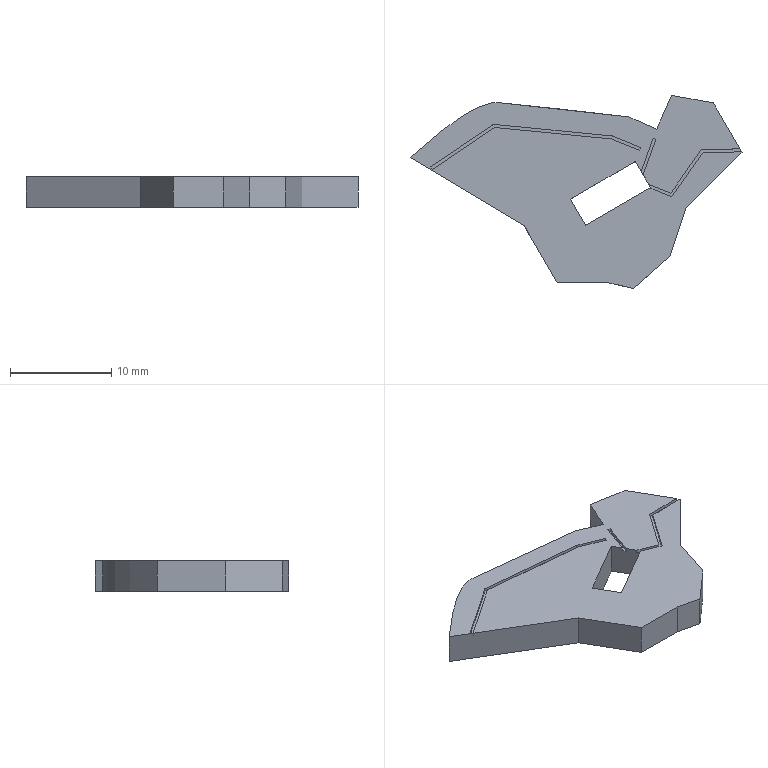Part | SolidWorks | features BaseBody 1 | 1 solid | 39 faces | box 32.789 x 19.083 x 3 mm | volume 1028 mm3 | plane 29 | spline 10
STEP:
#1=CARTESIAN_POINT('',(-62.576,-66.824,1.2));
#2=VERTEX_POINT('',#1);
#3=CARTESIAN_POINT('',(-68.833,-71.037,1.2));
#4=VERTEX_POINT('',#3);
#5=CARTESIAN_POINT('',(-62.665,-66.884,1.2));
#6=DIRECTION('',(-0.8295,-0.5585,0.));
#7=VECTOR('',#6,1000.);
#8=LINE('',#5,#7);
#9=EDGE_CURVE('',#2,#4,#8,.T.);
#10=ORIENTED_EDGE('',*,*,#9,.T.);
#11=CARTESIAN_POINT('',(-68.666,-71.286,1.2));
#12=VERTEX_POINT('',#11);
#13=CARTESIAN_POINT('',(-68.666,-71.286,1.2));
#14=DIRECTION('',(-0.5585,0.8295,0.));
#15=VECTOR('',#14,1000.);
#16=LINE('',#13,#15);
#17=EDGE_CURVE('',#12,#4,#16,.T.);
#18=ORIENTED_EDGE('',*,*,#17,.F.);
#19=CARTESIAN_POINT('',(-62.498,-67.133,1.2));
#20=VERTEX_POINT('',#19);
#21=CARTESIAN_POINT('',(-62.498,-67.133,1.2));
#22=DIRECTION('',(-0.8295,-0.5585,0.));
#23=VECTOR('',#22,1000.);
#24=LINE('',#21,#23);
#25=EDGE_CURVE('',#20,#12,#24,.T.);
#26=ORIENTED_EDGE('',*,*,#25,.F.);
#27=CARTESIAN_POINT('',(-50.939,-68.271,1.2));
#28=VERTEX_POINT('',#27);
#29=CARTESIAN_POINT('',(-50.939,-68.271,1.2));
#30=DIRECTION('',(-0.9952,0.09803,0.));
#31=VECTOR('',#30,1000.);
#32=LINE('',#29,#31);
#33=EDGE_CURVE('',#28,#20,#32,.T.);
#34=ORIENTED_EDGE('',*,*,#33,.F.);
#35=CARTESIAN_POINT('',(-48.164,-69.391,1.2));
#36=VERTEX_POINT('',#35);
#37=CARTESIAN_POINT('',(-48.164,-69.391,1.2));
#38=DIRECTION('',(-0.9274,0.3742,0.));
#39=VECTOR('',#38,1000.);
#40=LINE('',#37,#39);
#41=EDGE_CURVE('',#36,#28,#40,.T.);
#42=ORIENTED_EDGE('',*,*,#41,.F.);
#43=CARTESIAN_POINT('',(-48.051,-69.113,1.2));
#44=VERTEX_POINT('',#43);
#45=CARTESIAN_POINT('',(-48.051,-69.113,1.2));
#46=DIRECTION('',(-0.3742,-0.9274,0.));
#47=VECTOR('',#46,1000.);
#48=LINE('',#45,#47);
#49=EDGE_CURVE('',#44,#36,#48,.T.);
#50=ORIENTED_EDGE('',*,*,#49,.F.);
#51=CARTESIAN_POINT('',(-50.867,-67.977,1.2));
#52=VERTEX_POINT('',#51);
#53=CARTESIAN_POINT('',(-48.051,-69.113,1.2));
#54=DIRECTION('',(-0.9274,0.3742,0.));
#55=VECTOR('',#54,1000.);
#56=LINE('',#53,#55);
#57=EDGE_CURVE('',#44,#52,#56,.T.);
#58=ORIENTED_EDGE('',*,*,#57,.T.);
#59=CARTESIAN_POINT('',(-50.91,-67.973,1.2));
#60=DIRECTION('',(-0.9952,0.09803,0.));
#61=VECTOR('',#60,1000.);
#62=LINE('',#59,#61);
#63=EDGE_CURVE('',#52,#2,#62,.T.);
#64=ORIENTED_EDGE('',*,*,#63,.T.);
#65=EDGE_LOOP('',(#10,#18,#26,#34,#42,#50,#58,#64));
#66=FACE_OUTER_BOUND('',#65,.T.);
#67=CARTESIAN_POINT('',(0.,0.,1.2));
#68=DIRECTION('',(0.,0.,-1.));
#69=DIRECTION('',(0.,-1.,0.));
#70=AXIS2_PLACEMENT_3D('',#67,#68,#69);
#71=PLANE('',#70);
#72=ADVANCED_FACE('',(#66),#71,.F.);
#73=CARTESIAN_POINT('',(-68.666,-71.286,1.5));
#74=VERTEX_POINT('',#73);
#75=CARTESIAN_POINT('',(-68.833,-71.037,1.5));
#76=VERTEX_POINT('',#75);
#77=CARTESIAN_POINT('',(-68.666,-71.286,1.5));
#78=DIRECTION('',(-0.5585,0.8295,0.));
#79=VECTOR('',#78,1000.);
#80=LINE('',#77,#79);
#81=EDGE_CURVE('',#74,#76,#80,.T.);
#82=ORIENTED_EDGE('',*,*,#81,.F.);
#83=CARTESIAN_POINT('',(-68.666,-71.286,1.2));
#84=DIRECTION('',(0.,0.,1.));
#85=VECTOR('',#84,1000.);
#86=LINE('',#83,#85);
#87=EDGE_CURVE('',#12,#74,#86,.T.);
#88=ORIENTED_EDGE('',*,*,#87,.F.);
#89=ORIENTED_EDGE('',*,*,#17,.T.);
#90=CARTESIAN_POINT('',(-68.833,-71.037,1.2));
#91=DIRECTION('',(0.,0.,1.));
#92=VECTOR('',#91,1000.);
#93=LINE('',#90,#92);
#94=EDGE_CURVE('',#4,#76,#93,.T.);
#95=ORIENTED_EDGE('',*,*,#94,.T.);
#96=EDGE_LOOP('',(#82,#88,#89,#95));
#97=FACE_OUTER_BOUND('',#96,.T.);
#98=CARTESIAN_POINT('',(-68.666,-71.286,1.2));
#99=DIRECTION('',(0.8295,0.5585,0.));
#100=DIRECTION('',(0.,0.,-1.));
#101=AXIS2_PLACEMENT_3D('',#98,#99,#100);
#102=PLANE('',#101);
#103=ADVANCED_FACE('',(#97),#102,.T.);
#104=CARTESIAN_POINT('',(-62.498,-67.133,1.5));
#105=VERTEX_POINT('',#104);
#106=CARTESIAN_POINT('',(-62.498,-67.133,1.5));
#107=DIRECTION('',(-0.8295,-0.5585,0.));
#108=VECTOR('',#107,1000.);
#109=LINE('',#106,#108);
#110=EDGE_CURVE('',#105,#74,#109,.T.);
#111=ORIENTED_EDGE('',*,*,#110,.F.);
#112=CARTESIAN_POINT('',(-62.498,-67.133,1.2));
#113=DIRECTION('',(0.,0.,1.));
#114=VECTOR('',#113,1000.);
#115=LINE('',#112,#114);
#116=EDGE_CURVE('',#20,#105,#115,.T.);
#117=ORIENTED_EDGE('',*,*,#116,.F.);
#118=ORIENTED_EDGE('',*,*,#25,.T.);
#119=ORIENTED_EDGE('',*,*,#87,.T.);
#120=EDGE_LOOP('',(#111,#117,#118,#119));
#121=FACE_OUTER_BOUND('',#120,.T.);
#122=CARTESIAN_POINT('',(-62.498,-67.133,1.2));
#123=DIRECTION('',(-0.5585,0.8295,0.));
#124=DIRECTION('',(0.,0.,1.));
#125=AXIS2_PLACEMENT_3D('',#122,#123,#124);
#126=PLANE('',#125);
#127=ADVANCED_FACE('',(#121),#126,.T.);
#128=CARTESIAN_POINT('',(-50.939,-68.271,1.5));
#129=VERTEX_POINT('',#128);
#130=CARTESIAN_POINT('',(-50.939,-68.271,1.5));
#131=DIRECTION('',(-0.9952,0.09803,0.));
#132=VECTOR('',#131,1000.);
#133=LINE('',#130,#132);
#134=EDGE_CURVE('',#129,#105,#133,.T.);
#135=ORIENTED_EDGE('',*,*,#134,.F.);
#136=CARTESIAN_POINT('',(-50.939,-68.271,1.2));
#137=DIRECTION('',(0.,0.,1.));
#138=VECTOR('',#137,1000.);
#139=LINE('',#136,#138);
#140=EDGE_CURVE('',#28,#129,#139,.T.);
#141=ORIENTED_EDGE('',*,*,#140,.F.);
#142=ORIENTED_EDGE('',*,*,#33,.T.);
#143=ORIENTED_EDGE('',*,*,#116,.T.);
#144=EDGE_LOOP('',(#135,#141,#142,#143));
#145=FACE_OUTER_BOUND('',#144,.T.);
#146=CARTESIAN_POINT('',(-50.939,-68.271,1.2));
#147=DIRECTION('',(0.09803,0.9952,0.));
#148=DIRECTION('',(0.,0.,-1.));
#149=AXIS2_PLACEMENT_3D('',#146,#147,#148);
#150=PLANE('',#149);
#151=ADVANCED_FACE('',(#145),#150,.T.);
#152=CARTESIAN_POINT('',(-48.164,-69.391,1.5));
#153=VERTEX_POINT('',#152);
#154=CARTESIAN_POINT('',(-48.164,-69.391,1.5));
#155=DIRECTION('',(-0.9274,0.3742,0.));
#156=VECTOR('',#155,1000.);
#157=LINE('',#154,#156);
#158=EDGE_CURVE('',#153,#129,#157,.T.);
#159=ORIENTED_EDGE('',*,*,#158,.F.);
#160=CARTESIAN_POINT('',(-48.164,-69.391,1.2));
#161=DIRECTION('',(0.,0.,1.));
#162=VECTOR('',#161,1000.);
#163=LINE('',#160,#162);
#164=EDGE_CURVE('',#36,#153,#163,.T.);
#165=ORIENTED_EDGE('',*,*,#164,.F.);
#166=ORIENTED_EDGE('',*,*,#41,.T.);
#167=ORIENTED_EDGE('',*,*,#140,.T.);
#168=EDGE_LOOP('',(#159,#165,#166,#167));
#169=FACE_OUTER_BOUND('',#168,.T.);
#170=CARTESIAN_POINT('',(-48.164,-69.391,1.2));
#171=DIRECTION('',(0.3742,0.9274,0.));
#172=DIRECTION('',(0.,0.,-1.));
#173=AXIS2_PLACEMENT_3D('',#170,#171,#172);
#174=PLANE('',#173);
#175=ADVANCED_FACE('',(#169),#174,.T.);
#176=CARTESIAN_POINT('',(-48.051,-69.113,1.5));
#177=VERTEX_POINT('',#176);
#178=CARTESIAN_POINT('',(-48.051,-69.113,1.5));
#179=DIRECTION('',(-0.3742,-0.9274,0.));
#180=VECTOR('',#179,1000.);
#181=LINE('',#178,#180);
#182=EDGE_CURVE('',#177,#153,#181,.T.);
#183=ORIENTED_EDGE('',*,*,#182,.F.);
#184=CARTESIAN_POINT('',(-48.051,-69.113,1.2));
#185=DIRECTION('',(0.,0.,1.));
#186=VECTOR('',#185,1000.);
#187=LINE('',#184,#186);
#188=EDGE_CURVE('',#44,#177,#187,.T.);
#189=ORIENTED_EDGE('',*,*,#188,.F.);
#190=ORIENTED_EDGE('',*,*,#49,.T.);
#191=ORIENTED_EDGE('',*,*,#164,.T.);
#192=EDGE_LOOP('',(#183,#189,#190,#191));
#193=FACE_OUTER_BOUND('',#192,.T.);
#194=CARTESIAN_POINT('',(-48.051,-69.113,1.2));
#195=DIRECTION('',(-0.9274,0.3742,0.));
#196=DIRECTION('',(0.,0.,1.));
#197=AXIS2_PLACEMENT_3D('',#194,#195,#196);
#198=PLANE('',#197);
#199=ADVANCED_FACE('',(#193),#198,.T.);
#200=CARTESIAN_POINT('',(-50.867,-67.977,1.5));
#201=VERTEX_POINT('',#200);
#202=CARTESIAN_POINT('',(-48.051,-69.113,1.5));
#203=DIRECTION('',(-0.9274,0.3742,0.));
#204=VECTOR('',#203,1000.);
#205=LINE('',#202,#204);
#206=EDGE_CURVE('',#177,#201,#205,.T.);
#207=ORIENTED_EDGE('',*,*,#206,.T.);
#208=CARTESIAN_POINT('',(-50.867,-67.977,1.2));
#209=DIRECTION('',(0.,0.,1.));
#210=VECTOR('',#209,1000.);
#211=LINE('',#208,#210);
#212=EDGE_CURVE('',#52,#201,#211,.T.);
#213=ORIENTED_EDGE('',*,*,#212,.F.);
#214=ORIENTED_EDGE('',*,*,#57,.F.);
#215=ORIENTED_EDGE('',*,*,#188,.T.);
#216=EDGE_LOOP('',(#207,#213,#214,#215));
#217=FACE_OUTER_BOUND('',#216,.T.);
#218=CARTESIAN_POINT('',(-48.051,-69.113,1.2));
#219=DIRECTION('',(0.3742,0.9274,0.));
#220=DIRECTION('',(0.,0.,-1.));
#221=AXIS2_PLACEMENT_3D('',#218,#219,#220);
#222=PLANE('',#221);
#223=ADVANCED_FACE('',(#217),#222,.F.);
#224=CARTESIAN_POINT('',(-62.576,-66.824,1.5));
#225=VERTEX_POINT('',#224);
#226=CARTESIAN_POINT('',(-50.91,-67.973,1.5));
#227=DIRECTION('',(-0.9952,0.09803,0.));
#228=VECTOR('',#227,1000.);
#229=LINE('',#226,#228);
#230=EDGE_CURVE('',#201,#225,#229,.T.);
#231=ORIENTED_EDGE('',*,*,#230,.T.);
#232=CARTESIAN_POINT('',(-62.576,-66.824,1.2));
#233=DIRECTION('',(0.,0.,1.));
#234=VECTOR('',#233,1000.);
#235=LINE('',#232,#234);
#236=EDGE_CURVE('',#2,#225,#235,.T.);
#237=ORIENTED_EDGE('',*,*,#236,.F.);
#238=ORIENTED_EDGE('',*,*,#63,.F.);
#239=ORIENTED_EDGE('',*,*,#212,.T.);
#240=EDGE_LOOP('',(#231,#237,#238,#239));
#241=FACE_OUTER_BOUND('',#240,.T.);
#242=CARTESIAN_POINT('',(-50.91,-67.973,1.2));
#243=DIRECTION('',(0.09803,0.9952,0.));
#244=DIRECTION('',(0.,0.,-1.));
#245=AXIS2_PLACEMENT_3D('',#242,#243,#244);
#246=PLANE('',#245);
#247=ADVANCED_FACE('',(#241),#246,.F.);
#248=CARTESIAN_POINT('',(-62.665,-66.884,1.5));
#249=DIRECTION('',(-0.8295,-0.5585,0.));
#250=VECTOR('',#249,1000.);
#251=LINE('',#248,#250);
#252=EDGE_CURVE('',#225,#76,#251,.T.);
#253=ORIENTED_EDGE('',*,*,#252,.T.);
#254=ORIENTED_EDGE('',*,*,#94,.F.);
#255=ORIENTED_EDGE('',*,*,#9,.F.);
#256=ORIENTED_EDGE('',*,*,#236,.T.);
#257=EDGE_LOOP('',(#253,#254,#255,#256));
#258=FACE_OUTER_BOUND('',#257,.T.);
#259=CARTESIAN_POINT('',(-62.665,-66.884,1.2));
#260=DIRECTION('',(-0.5585,0.8295,0.));
#261=DIRECTION('',(0.,0.,1.));
#262=AXIS2_PLACEMENT_3D('',#259,#260,#261);
#263=PLANE('',#262);
#264=ADVANCED_FACE('',(#258),#263,.F.);
#265=CARTESIAN_POINT('',(-41.906,-69.624,1.5));
#266=VERTEX_POINT('',#265);
#267=CARTESIAN_POINT('',(-44.985,-73.982,1.5));
#268=VERTEX_POINT('',#267);
#269=CARTESIAN_POINT('',(-41.906,-69.624,1.5));
#270=DIRECTION('',(-0.5771,-0.8167,0.));
#271=VECTOR('',#270,1000.);
#272=LINE('',#269,#271);
#273=EDGE_CURVE('',#266,#268,#272,.T.);
#274=ORIENTED_EDGE('',*,*,#273,.F.);
#275=CARTESIAN_POINT('',(-41.906,-69.624,1.2));
#276=VERTEX_POINT('',#275);
#277=CARTESIAN_POINT('',(-41.906,-69.624,1.2));
#278=DIRECTION('',(0.,0.,1.));
#279=VECTOR('',#278,1000.);
#280=LINE('',#277,#279);
#281=EDGE_CURVE('',#276,#266,#280,.T.);
#282=ORIENTED_EDGE('',*,*,#281,.F.);
#283=CARTESIAN_POINT('',(-44.985,-73.982,1.2));
#284=VERTEX_POINT('',#283);
#285=CARTESIAN_POINT('',(-41.906,-69.624,1.2));
#286=DIRECTION('',(-0.5771,-0.8167,0.));
#287=VECTOR('',#286,1000.);
#288=LINE('',#285,#287);
#289=EDGE_CURVE('',#276,#284,#288,.T.);
#290=ORIENTED_EDGE('',*,*,#289,.T.);
#291=CARTESIAN_POINT('',(-44.985,-73.982,1.2));
#292=DIRECTION('',(0.,0.,1.));
#293=VECTOR('',#292,1000.);
#294=LINE('',#291,#293);
#295=EDGE_CURVE('',#284,#268,#294,.T.);
#296=ORIENTED_EDGE('',*,*,#295,.T.);
#297=EDGE_LOOP('',(#274,#282,#290,#296));
#298=FACE_OUTER_BOUND('',#297,.T.);
#299=CARTESIAN_POINT('',(-41.906,-69.624,1.2));
#300=DIRECTION('',(-0.8167,0.5771,0.));
#301=DIRECTION('',(0.,0.,1.));
#302=AXIS2_PLACEMENT_3D('',#299,#300,#301);
#303=PLANE('',#302);
#304=ADVANCED_FACE('',(#298),#303,.T.);
#305=CARTESIAN_POINT('',(-42.063,-69.328,1.5));
#306=VERTEX_POINT('',#305);
#307=CARTESIAN_POINT('',(-45.093,-73.616,1.5));
#308=VERTEX_POINT('',#307);
#309=CARTESIAN_POINT('',(-42.151,-69.451,1.5));
#310=DIRECTION('',(-0.5771,-0.8167,0.));
#311=VECTOR('',#310,1000.);
#312=LINE('',#309,#311);
#313=EDGE_CURVE('',#306,#308,#312,.T.);
#314=ORIENTED_EDGE('',*,*,#313,.T.);
#315=CARTESIAN_POINT('',(-45.093,-73.616,1.2));
#316=VERTEX_POINT('',#315);
#317=CARTESIAN_POINT('',(-45.093,-73.616,1.2));
#318=DIRECTION('',(0.,0.,1.));
#319=VECTOR('',#318,1000.);
#320=LINE('',#317,#319);
#321=EDGE_CURVE('',#316,#308,#320,.T.);
#322=ORIENTED_EDGE('',*,*,#321,.F.);
#323=CARTESIAN_POINT('',(-42.063,-69.328,1.2));
#324=VERTEX_POINT('',#323);
#325=CARTESIAN_POINT('',(-42.151,-69.451,1.2));
#326=DIRECTION('',(-0.5771,-0.8167,0.));
#327=VECTOR('',#326,1000.);
#328=LINE('',#325,#327);
#329=EDGE_CURVE('',#324,#316,#328,.T.);
#330=ORIENTED_EDGE('',*,*,#329,.F.);
#331=CARTESIAN_POINT('',(-42.063,-69.328,1.2));
#332=DIRECTION('',(0.,0.,1.));
#333=VECTOR('',#332,1000.);
#334=LINE('',#331,#333);
#335=EDGE_CURVE('',#324,#306,#334,.T.);
#336=ORIENTED_EDGE('',*,*,#335,.T.);
#337=EDGE_LOOP('',(#314,#322,#330,#336));
#338=FACE_OUTER_BOUND('',#337,.T.);
#339=CARTESIAN_POINT('',(-42.151,-69.451,1.2));
#340=DIRECTION('',(-0.8167,0.5771,0.));
#341=DIRECTION('',(0.,0.,1.));
#342=AXIS2_PLACEMENT_3D('',#339,#340,#341);
#343=PLANE('',#342);
#344=ADVANCED_FACE('',(#338),#343,.F.);
#345=CARTESIAN_POINT('',(-47.153,-73.119,1.2));
#346=VERTEX_POINT('',#345);
#347=CARTESIAN_POINT('',(-47.153,-73.119,1.5));
#348=VERTEX_POINT('',#347);
#349=CARTESIAN_POINT('',(-47.153,-73.119,-1.5));
#350=DIRECTION('',(0.,0.,1.));
#351=VECTOR('',#350,1000.);
#352=LINE('',#349,#351);
#353=EDGE_CURVE('',#346,#348,#352,.T.);
#354=ORIENTED_EDGE('',*,*,#353,.T.);
#355=CARTESIAN_POINT('',(-44.985,-73.982,1.5));
#356=DIRECTION('',(-0.9292,0.3696,0.));
#357=VECTOR('',#356,1000.);
#358=LINE('',#355,#357);
#359=EDGE_CURVE('',#268,#348,#358,.T.);
#360=ORIENTED_EDGE('',*,*,#359,.F.);
#361=ORIENTED_EDGE('',*,*,#295,.F.);
#362=CARTESIAN_POINT('',(-44.985,-73.982,1.2));
#363=DIRECTION('',(-0.9292,0.3696,0.));
#364=VECTOR('',#363,1000.);
#365=LINE('',#362,#364);
#366=EDGE_CURVE('',#284,#346,#365,.T.);
#367=ORIENTED_EDGE('',*,*,#366,.T.);
#368=EDGE_LOOP('',(#354,#360,#361,#367));
#369=FACE_OUTER_BOUND('',#368,.T.);
#370=CARTESIAN_POINT('',(-44.985,-73.982,1.2));
#371=DIRECTION('',(0.3696,0.9292,0.));
#372=DIRECTION('',(0.,0.,-1.));
#373=AXIS2_PLACEMENT_3D('',#370,#371,#372);
#374=PLANE('',#373);
#375=ADVANCED_FACE('',(#369),#374,.T.);
#376=CARTESIAN_POINT('',(-38.1,-69.542,1.5));
#377=VERTEX_POINT('',#376);
#378=CARTESIAN_POINT('',(-38.1,-69.542,1.2));
#379=VERTEX_POINT('',#378);
#380=CARTESIAN_POINT('',(-38.1,-69.542,-1.5));
#381=DIRECTION('',(0.,0.,-1.));
#382=VECTOR('',#381,1000.);
#383=LINE('',#380,#382);
#384=EDGE_CURVE('',#377,#379,#383,.T.);
#385=ORIENTED_EDGE('',*,*,#384,.T.);
#386=CARTESIAN_POINT('',(-35.474,-69.486,1.2));
#387=DIRECTION('',(-0.9998,-0.02153,0.));
#388=VECTOR('',#387,1000.);
#389=LINE('',#386,#388);
#390=EDGE_CURVE('',#379,#276,#389,.T.);
#391=ORIENTED_EDGE('',*,*,#390,.T.);
#392=ORIENTED_EDGE('',*,*,#281,.T.);
#393=CARTESIAN_POINT('',(1.479,-68.69,1.5));
#394=DIRECTION('',(-0.9998,-0.02153,0.));
#395=VECTOR('',#394,1000.);
#396=LINE('',#393,#395);
#397=EDGE_CURVE('',#377,#266,#396,.T.);
#398=ORIENTED_EDGE('',*,*,#397,.F.);
#399=EDGE_LOOP('',(#385,#391,#392,#398));
#400=FACE_OUTER_BOUND('',#399,.T.);
#401=CARTESIAN_POINT('',(-35.474,-69.486,1.2));
#402=DIRECTION('',(-0.02153,0.9998,0.));
#403=DIRECTION('',(0.,0.,1.));
#404=AXIS2_PLACEMENT_3D('',#401,#402,#403);
#405=PLANE('',#404);
#406=ADVANCED_FACE('',(#400),#405,.T.);
#407=CARTESIAN_POINT('',(-38.271,-69.246,1.5));
#408=VERTEX_POINT('',#407);
#409=CARTESIAN_POINT('',(1.473,-68.39,1.5));
#410=DIRECTION('',(-0.9998,-0.02153,0.));
#411=VECTOR('',#410,1000.);
#412=LINE('',#409,#411);
#413=EDGE_CURVE('',#408,#306,#412,.T.);
#414=ORIENTED_EDGE('',*,*,#413,.T.);
#415=ORIENTED_EDGE('',*,*,#335,.F.);
#416=CARTESIAN_POINT('',(-38.271,-69.246,1.2));
#417=VERTEX_POINT('',#416);
#418=CARTESIAN_POINT('',(-35.481,-69.186,1.2));
#419=DIRECTION('',(-0.9998,-0.02153,0.));
#420=VECTOR('',#419,1000.);
#421=LINE('',#418,#420);
#422=EDGE_CURVE('',#417,#324,#421,.T.);
#423=ORIENTED_EDGE('',*,*,#422,.F.);
#424=CARTESIAN_POINT('',(-38.271,-69.246,-1.5));
#425=DIRECTION('',(0.,0.,-1.));
#426=VECTOR('',#425,1000.);
#427=LINE('',#424,#426);
#428=EDGE_CURVE('',#408,#417,#427,.T.);
#429=ORIENTED_EDGE('',*,*,#428,.F.);
#430=EDGE_LOOP('',(#414,#415,#423,#429));
#431=FACE_OUTER_BOUND('',#430,.T.);
#432=CARTESIAN_POINT('',(-35.481,-69.186,1.2));
#433=DIRECTION('',(-0.02153,0.9998,0.));
#434=DIRECTION('',(0.,0.,1.));
#435=AXIS2_PLACEMENT_3D('',#432,#433,#434);
#436=PLANE('',#435);
#437=ADVANCED_FACE('',(#431),#436,.F.);
#438=CARTESIAN_POINT('',(-47.269,-72.75,1.2));
#439=VERTEX_POINT('',#438);
#440=CARTESIAN_POINT('',(-44.874,-73.703,1.2));
#441=DIRECTION('',(-0.9292,0.3696,0.));
#442=VECTOR('',#441,1000.);
#443=LINE('',#440,#442);
#444=EDGE_CURVE('',#316,#439,#443,.T.);
#445=ORIENTED_EDGE('',*,*,#444,.F.);
#446=ORIENTED_EDGE('',*,*,#321,.T.);
#447=CARTESIAN_POINT('',(-47.269,-72.75,1.5));
#448=VERTEX_POINT('',#447);
#449=CARTESIAN_POINT('',(-44.874,-73.703,1.5));
#450=DIRECTION('',(-0.9292,0.3696,0.));
#451=VECTOR('',#450,1000.);
#452=LINE('',#449,#451);
#453=EDGE_CURVE('',#308,#448,#452,.T.);
#454=ORIENTED_EDGE('',*,*,#453,.T.);
#455=CARTESIAN_POINT('',(-47.269,-72.75,-1.5));
#456=DIRECTION('',(0.,0.,1.));
#457=VECTOR('',#456,1000.);
#458=LINE('',#455,#457);
#459=EDGE_CURVE('',#439,#448,#458,.T.);
#460=ORIENTED_EDGE('',*,*,#459,.F.);
#461=EDGE_LOOP('',(#445,#446,#454,#460));
#462=FACE_OUTER_BOUND('',#461,.T.);
#463=CARTESIAN_POINT('',(-44.874,-73.703,1.2));
#464=DIRECTION('',(0.3696,0.9292,0.));
#465=DIRECTION('',(0.,0.,-1.));
#466=AXIS2_PLACEMENT_3D('',#463,#464,#465);
#467=PLANE('',#466);
#468=ADVANCED_FACE('',(#462),#467,.F.);
#469=ORIENTED_EDGE('',*,*,#422,.T.);
#470=ORIENTED_EDGE('',*,*,#329,.T.);
#471=ORIENTED_EDGE('',*,*,#444,.T.);
#472=CARTESIAN_POINT('',(-47.079,-73.076,1.2));
#473=VERTEX_POINT('',#472);
#474=CARTESIAN_POINT('',(-66.934,-38.993,1.2));
#475=DIRECTION('',(-0.5034,0.8641,0.));
#476=VECTOR('',#475,1000.);
#477=LINE('',#474,#476);
#478=EDGE_CURVE('',#473,#439,#477,.T.);
#479=ORIENTED_EDGE('',*,*,#478,.F.);
#480=CARTESIAN_POINT('',(19.855,-34.083,1.2));
#481=DIRECTION('',(0.8641,0.5034,0.));
#482=VECTOR('',#481,1000.);
#483=LINE('',#480,#482);
#484=EDGE_CURVE('',#346,#473,#483,.T.);
#485=ORIENTED_EDGE('',*,*,#484,.F.);
#486=ORIENTED_EDGE('',*,*,#366,.F.);
#487=ORIENTED_EDGE('',*,*,#289,.F.);
#488=ORIENTED_EDGE('',*,*,#390,.F.);
#489=CARTESIAN_POINT('',(-38.271,-69.246,1.2));
#490=CARTESIAN_POINT('',(-38.214,-69.345,1.2));
#491=CARTESIAN_POINT('',(-38.157,-69.444,1.2));
#492=CARTESIAN_POINT('',(-38.1,-69.542,1.2));
#493=B_SPLINE_CURVE_WITH_KNOTS('',3,(#489,#490,#491,#492),.UNSPECIFIED.,.F.,.F.,(4,4),(0.07694,0.07936),.UNSPECIFIED.);
#494=EDGE_CURVE('',#417,#379,#493,.T.);
#495=ORIENTED_EDGE('',*,*,#494,.F.);
#496=EDGE_LOOP('',(#469,#470,#471,#479,#485,#486,#487,#488,#495));
#497=FACE_OUTER_BOUND('',#496,.T.);
#498=CARTESIAN_POINT('',(0.,0.,1.2));
#499=DIRECTION('',(0.,0.,-1.));
#500=DIRECTION('',(0.,-1.,0.));
#501=AXIS2_PLACEMENT_3D('',#498,#499,#500);
#502=PLANE('',#501);
#503=ADVANCED_FACE('',(#497),#502,.F.);
#504=CARTESIAN_POINT('',(-47.815,-71.813,1.2));
#505=VERTEX_POINT('',#504);
#506=CARTESIAN_POINT('',(-46.56,-68.307,1.2));
#507=VERTEX_POINT('',#506);
#508=CARTESIAN_POINT('',(-48.138,-72.716,1.2));
#509=DIRECTION('',(0.337,0.9415,0.));
#510=VECTOR('',#509,1000.);
#511=LINE('',#508,#510);
#512=EDGE_CURVE('',#505,#507,#511,.T.);
#513=ORIENTED_EDGE('',*,*,#512,.T.);
#514=CARTESIAN_POINT('',(-46.843,-68.206,1.2));
#515=VERTEX_POINT('',#514);
#516=CARTESIAN_POINT('',(-46.843,-68.206,1.2));
#517=DIRECTION('',(0.9415,-0.337,0.));
#518=VECTOR('',#517,1000.);
#519=LINE('',#516,#518);
#520=EDGE_CURVE('',#515,#507,#519,.T.);
#521=ORIENTED_EDGE('',*,*,#520,.F.);
#522=CARTESIAN_POINT('',(-48.012,-71.474,1.2));
#523=VERTEX_POINT('',#522);
#524=CARTESIAN_POINT('',(-48.42,-72.615,1.2));
#525=DIRECTION('',(0.337,0.9415,0.));
#526=VECTOR('',#525,1000.);
#527=LINE('',#524,#526);
#528=EDGE_CURVE('',#523,#515,#527,.T.);
#529=ORIENTED_EDGE('',*,*,#528,.F.);
#530=CARTESIAN_POINT('',(-66.934,-38.993,1.2));
#531=DIRECTION('',(-0.5034,0.8641,0.));
#532=VECTOR('',#531,1000.);
#533=LINE('',#530,#532);
#534=EDGE_CURVE('',#505,#523,#533,.T.);
#535=ORIENTED_EDGE('',*,*,#534,.F.);
#536=EDGE_LOOP('',(#513,#521,#529,#535));
#537=FACE_OUTER_BOUND('',#536,.T.);
#538=CARTESIAN_POINT('',(0.,0.,1.2));
#539=DIRECTION('',(0.,0.,-1.));
#540=DIRECTION('',(0.,-1.,0.));
#541=AXIS2_PLACEMENT_3D('',#538,#539,#540);
#542=PLANE('',#541);
#543=ADVANCED_FACE('',(#537),#542,.F.);
#544=CARTESIAN_POINT('',(-47.815,-71.813,1.5));
#545=VERTEX_POINT('',#544);
#546=CARTESIAN_POINT('',(-46.56,-68.307,1.5));
#547=VERTEX_POINT('',#546);
#548=CARTESIAN_POINT('',(-19.604,7.016,1.5));
#549=DIRECTION('',(0.337,0.9415,0.));
#550=VECTOR('',#549,1000.);
#551=LINE('',#548,#550);
#552=EDGE_CURVE('',#545,#547,#551,.T.);
#553=ORIENTED_EDGE('',*,*,#552,.T.);
#554=CARTESIAN_POINT('',(-46.56,-68.307,1.2));
#555=DIRECTION('',(0.,0.,1.));
#556=VECTOR('',#555,1000.);
#557=LINE('',#554,#556);
#558=EDGE_CURVE('',#507,#547,#557,.T.);
#559=ORIENTED_EDGE('',*,*,#558,.F.);
#560=ORIENTED_EDGE('',*,*,#512,.F.);
#561=CARTESIAN_POINT('',(-47.815,-71.813,-1.5));
#562=DIRECTION('',(0.,0.,-1.));
#563=VECTOR('',#562,1000.);
#564=LINE('',#561,#563);
#565=EDGE_CURVE('',#545,#505,#564,.T.);
#566=ORIENTED_EDGE('',*,*,#565,.F.);
#567=EDGE_LOOP('',(#553,#559,#560,#566));
#568=FACE_OUTER_BOUND('',#567,.T.);
#569=CARTESIAN_POINT('',(-48.138,-72.716,1.2));
#570=DIRECTION('',(0.9415,-0.337,0.));
#571=DIRECTION('',(0.,0.,-1.));
#572=AXIS2_PLACEMENT_3D('',#569,#570,#571);
#573=PLANE('',#572);
#574=ADVANCED_FACE('',(#568),#573,.F.);
#575=CARTESIAN_POINT('',(-48.012,-71.474,1.5));
#576=VERTEX_POINT('',#575);
#577=CARTESIAN_POINT('',(-48.012,-71.474,-1.5));
#578=DIRECTION('',(0.,0.,-1.));
#579=VECTOR('',#578,1000.);
#580=LINE('',#577,#579);
#581=EDGE_CURVE('',#576,#523,#580,.T.);
#582=ORIENTED_EDGE('',*,*,#581,.T.);
#583=ORIENTED_EDGE('',*,*,#528,.T.);
#584=CARTESIAN_POINT('',(-46.843,-68.206,1.5));
#585=VERTEX_POINT('',#584);
#586=CARTESIAN_POINT('',(-46.843,-68.206,1.2));
#587=DIRECTION('',(0.,0.,1.));
#588=VECTOR('',#587,1000.);
#589=LINE('',#586,#588);
#590=EDGE_CURVE('',#515,#585,#589,.T.);
#591=ORIENTED_EDGE('',*,*,#590,.T.);
#592=CARTESIAN_POINT('',(-19.886,7.117,1.5));
#593=DIRECTION('',(0.337,0.9415,0.));
#594=VECTOR('',#593,1000.);
#595=LINE('',#592,#594);
#596=EDGE_CURVE('',#576,#585,#595,.T.);
#597=ORIENTED_EDGE('',*,*,#596,.F.);
#598=EDGE_LOOP('',(#582,#583,#591,#597));
#599=FACE_OUTER_BOUND('',#598,.T.);
#600=CARTESIAN_POINT('',(-48.42,-72.615,1.2));
#601=DIRECTION('',(0.9415,-0.337,0.));
#602=DIRECTION('',(0.,0.,-1.));
#603=AXIS2_PLACEMENT_3D('',#600,#601,#602);
#604=PLANE('',#603);
#605=ADVANCED_FACE('',(#599),#604,.T.);
#606=CARTESIAN_POINT('',(-46.843,-68.206,1.5));
#607=DIRECTION('',(0.9415,-0.337,0.));
#608=VECTOR('',#607,1000.);
#609=LINE('',#606,#608);
#610=EDGE_CURVE('',#585,#547,#609,.T.);
#611=ORIENTED_EDGE('',*,*,#610,.F.);
#612=ORIENTED_EDGE('',*,*,#590,.F.);
#613=ORIENTED_EDGE('',*,*,#520,.T.);
#614=ORIENTED_EDGE('',*,*,#558,.T.);
#615=EDGE_LOOP('',(#611,#612,#613,#614));
#616=FACE_OUTER_BOUND('',#615,.T.);
#617=CARTESIAN_POINT('',(-46.843,-68.206,1.2));
#618=DIRECTION('',(-0.337,-0.9415,0.));
#619=DIRECTION('',(-0.9415,0.337,0.));
#620=AXIS2_PLACEMENT_3D('',#617,#618,#619);
#621=PLANE('',#620);
#622=ADVANCED_FACE('',(#616),#621,.T.);
#623=ORIENTED_EDGE('',*,*,#252,.F.);
#624=ORIENTED_EDGE('',*,*,#230,.F.);
#625=ORIENTED_EDGE('',*,*,#206,.F.);
#626=ORIENTED_EDGE('',*,*,#182,.T.);
#627=ORIENTED_EDGE('',*,*,#158,.T.);
#628=ORIENTED_EDGE('',*,*,#134,.T.);
#629=ORIENTED_EDGE('',*,*,#110,.T.);
#630=ORIENTED_EDGE('',*,*,#81,.T.);
#631=EDGE_LOOP('',(#623,#624,#625,#626,#627,#628,#629,#630));
#632=FACE_BOUND('',#631,.T.);
#633=ORIENTED_EDGE('',*,*,#453,.F.);
#634=ORIENTED_EDGE('',*,*,#313,.F.);
#635=ORIENTED_EDGE('',*,*,#413,.F.);
#636=CARTESIAN_POINT('',(-40.879,-64.709,1.5));
#637=VERTEX_POINT('',#636);
#638=CARTESIAN_POINT('',(-40.879,-64.709,1.5));
#639=CARTESIAN_POINT('',(-40.008,-66.221,1.5));
#640=CARTESIAN_POINT('',(-39.141,-67.734,1.5));
#641=CARTESIAN_POINT('',(-38.271,-69.246,1.5));
#642=B_SPLINE_CURVE_WITH_KNOTS('',3,(#638,#639,#640,#641),.UNSPECIFIED.,.F.,.F.,(4,4),(0.04,0.07694),.UNSPECIFIED.);
#643=EDGE_CURVE('',#637,#408,#642,.T.);
#644=ORIENTED_EDGE('',*,*,#643,.F.);
#645=CARTESIAN_POINT('',(-45.006,-63.964,1.5));
#646=VERTEX_POINT('',#645);
#647=CARTESIAN_POINT('',(-45.006,-63.964,1.5));
#648=CARTESIAN_POINT('',(-43.631,-64.214,1.5));
#649=CARTESIAN_POINT('',(-42.255,-64.462,1.5));
#650=CARTESIAN_POINT('',(-40.879,-64.709,1.5));
#651=B_SPLINE_CURVE_WITH_KNOTS('',3,(#647,#648,#649,#650),.UNSPECIFIED.,.F.,.F.,(4,4),(0.00000001,0.04),.UNSPECIFIED.);
#652=EDGE_CURVE('',#646,#637,#651,.T.);
#653=ORIENTED_EDGE('',*,*,#652,.F.);
#654=CARTESIAN_POINT('',(-46.488,-67.303,1.5));
#655=VERTEX_POINT('',#654);
#656=CARTESIAN_POINT('',(-13.895,6.164,1.5));
#657=DIRECTION('',(-0.4055,-0.9141,0.));
#658=VECTOR('',#657,1000.);
#659=LINE('',#656,#658);
#660=EDGE_CURVE('',#646,#655,#659,.T.);
#661=ORIENTED_EDGE('',*,*,#660,.T.);
#662=CARTESIAN_POINT('',(-49.226,-66.088,1.5));
#663=VERTEX_POINT('',#662);
#664=CARTESIAN_POINT('',(-32.592,-73.468,1.5));
#665=DIRECTION('',(-0.9141,0.4055,0.));
#666=VECTOR('',#665,1000.);
#667=LINE('',#664,#666);
#668=EDGE_CURVE('',#655,#663,#667,.T.);
#669=ORIENTED_EDGE('',*,*,#668,.T.);
#670=CARTESIAN_POINT('',(-62.088,-64.682,1.5));
#671=VERTEX_POINT('',#670);
#672=CARTESIAN_POINT('',(-62.088,-64.682,1.5));
#673=CARTESIAN_POINT('',(-58.494,-65.013,1.5));
#674=CARTESIAN_POINT('',(-53.861,-65.551,1.5));
#675=CARTESIAN_POINT('',(-49.226,-66.088,1.5));
#676=B_SPLINE_CURVE_WITH_KNOTS('',3,(#672,#673,#674,#675),.UNSPECIFIED.,.F.,.F.,(4,4),(1.36,1.4),.UNSPECIFIED.);
#677=EDGE_CURVE('',#671,#663,#676,.T.);
#678=ORIENTED_EDGE('',*,*,#677,.F.);
#679=CARTESIAN_POINT('',(-70.844,-70.094,1.5));
#680=VERTEX_POINT('',#679);
#681=CARTESIAN_POINT('',(-70.844,-70.094,1.5));
#682=CARTESIAN_POINT('',(-67.569,-67.288,1.5));
#683=CARTESIAN_POINT('',(-64.295,-64.477,1.5));
#684=CARTESIAN_POINT('',(-62.088,-64.682,1.5));
#685=B_SPLINE_CURVE_WITH_KNOTS('',3,(#681,#682,#683,#684),.UNSPECIFIED.,.F.,.F.,(4,4),(1.32,1.36),.UNSPECIFIED.);
#686=EDGE_CURVE('',#680,#671,#685,.T.);
#687=ORIENTED_EDGE('',*,*,#686,.F.);
#688=CARTESIAN_POINT('',(-59.554,-76.86,1.5));
#689=VERTEX_POINT('',#688);
#690=CARTESIAN_POINT('',(-49.627,-82.809,1.5));
#691=DIRECTION('',(-0.8578,0.514,0.));
#692=VECTOR('',#691,1000.);
#693=LINE('',#690,#692);
#694=EDGE_CURVE('',#689,#680,#693,.T.);
#695=ORIENTED_EDGE('',*,*,#694,.F.);
#696=CARTESIAN_POINT('',(-56.318,-82.427,1.5));
#697=VERTEX_POINT('',#696);
#698=CARTESIAN_POINT('',(-56.318,-82.427,1.5));
#699=CARTESIAN_POINT('',(-57.397,-80.571,1.5));
#700=CARTESIAN_POINT('',(-58.477,-78.716,1.5));
#701=CARTESIAN_POINT('',(-59.554,-76.86,1.5));
#702=B_SPLINE_CURVE_WITH_KNOTS('',3,(#698,#699,#700,#701),.UNSPECIFIED.,.F.,.F.,(4,4),(0.28,0.32),.UNSPECIFIED.);
#703=EDGE_CURVE('',#697,#689,#702,.T.);
#704=ORIENTED_EDGE('',*,*,#703,.F.);
#705=CARTESIAN_POINT('',(-51.299,-82.456,1.5));
#706=VERTEX_POINT('',#705);
#707=CARTESIAN_POINT('',(-51.299,-82.456,1.5));
#708=CARTESIAN_POINT('',(-52.972,-82.448,1.5));
#709=CARTESIAN_POINT('',(-54.645,-82.437,1.5));
#710=CARTESIAN_POINT('',(-56.318,-82.427,1.5));
#711=B_SPLINE_CURVE_WITH_KNOTS('',3,(#707,#708,#709,#710),.UNSPECIFIED.,.F.,.F.,(4,4),(0.24,0.28),.UNSPECIFIED.);
#712=EDGE_CURVE('',#706,#697,#711,.T.);
#713=ORIENTED_EDGE('',*,*,#712,.F.);
#714=CARTESIAN_POINT('',(-48.767,-83.047,1.5));
#715=VERTEX_POINT('',#714);
#716=CARTESIAN_POINT('',(-48.767,-83.047,1.5));
#717=CARTESIAN_POINT('',(-49.611,-82.851,1.5));
#718=CARTESIAN_POINT('',(-50.455,-82.654,1.5));
#719=CARTESIAN_POINT('',(-51.299,-82.456,1.5));
#720=B_SPLINE_CURVE_WITH_KNOTS('',3,(#716,#717,#718,#719),.UNSPECIFIED.,.F.,.F.,(4,4),(0.2,0.24),.UNSPECIFIED.);
#721=EDGE_CURVE('',#715,#706,#720,.T.);
#722=ORIENTED_EDGE('',*,*,#721,.F.);
#723=CARTESIAN_POINT('',(-45.172,-79.871,1.5));
#724=VERTEX_POINT('',#723);
#725=CARTESIAN_POINT('',(-45.172,-79.871,1.5));
#726=CARTESIAN_POINT('',(-46.372,-80.932,1.5));
#727=CARTESIAN_POINT('',(-47.568,-81.988,1.5));
#728=CARTESIAN_POINT('',(-48.767,-83.047,1.5));
#729=B_SPLINE_CURVE_WITH_KNOTS('',3,(#725,#726,#727,#728),.UNSPECIFIED.,.F.,.F.,(4,4),(0.16,0.2),.UNSPECIFIED.);
#730=EDGE_CURVE('',#724,#715,#729,.T.);
#731=ORIENTED_EDGE('',*,*,#730,.F.);
#732=CARTESIAN_POINT('',(-43.587,-75.099,1.5));
#733=VERTEX_POINT('',#732);
#734=CARTESIAN_POINT('',(-43.587,-75.099,1.5));
#735=CARTESIAN_POINT('',(-44.115,-76.69,1.5));
#736=CARTESIAN_POINT('',(-44.644,-78.28,1.5));
#737=CARTESIAN_POINT('',(-45.172,-79.871,1.5));
#738=B_SPLINE_CURVE_WITH_KNOTS('',3,(#734,#735,#736,#737),.UNSPECIFIED.,.F.,.F.,(4,4),(0.12,0.16),.UNSPECIFIED.);
#739=EDGE_CURVE('',#733,#724,#738,.T.);
#740=ORIENTED_EDGE('',*,*,#739,.F.);
#741=CARTESIAN_POINT('',(-38.055,-69.621,1.5));
#742=VERTEX_POINT('',#741);
#743=CARTESIAN_POINT('',(-38.055,-69.621,1.5));
#744=CARTESIAN_POINT('',(-39.9,-71.449,1.5));
#745=CARTESIAN_POINT('',(-41.744,-73.272,1.5));
#746=CARTESIAN_POINT('',(-43.587,-75.099,1.5));
#747=B_SPLINE_CURVE_WITH_KNOTS('',3,(#743,#744,#745,#746),.UNSPECIFIED.,.F.,.F.,(4,4),(0.08,0.12),.UNSPECIFIED.);
#748=EDGE_CURVE('',#742,#733,#747,.T.);
#749=ORIENTED_EDGE('',*,*,#748,.F.);
#750=CARTESIAN_POINT('',(-38.1,-69.542,1.5));
#751=CARTESIAN_POINT('',(-38.085,-69.569,1.5));
#752=CARTESIAN_POINT('',(-38.07,-69.595,1.5));
#753=CARTESIAN_POINT('',(-38.055,-69.621,1.5));
#754=B_SPLINE_CURVE_WITH_KNOTS('',3,(#750,#751,#752,#753),.UNSPECIFIED.,.F.,.F.,(4,4),(0.07936,0.08),.UNSPECIFIED.);
#755=EDGE_CURVE('',#377,#742,#754,.T.);
#756=ORIENTED_EDGE('',*,*,#755,.F.);
#757=ORIENTED_EDGE('',*,*,#397,.T.);
#758=ORIENTED_EDGE('',*,*,#273,.T.);
#759=ORIENTED_EDGE('',*,*,#359,.T.);
#760=CARTESIAN_POINT('',(-53.48,-76.805,1.5));
#761=VERTEX_POINT('',#760);
#762=CARTESIAN_POINT('',(19.855,-34.083,1.5));
#763=DIRECTION('',(0.8641,0.5034,0.));
#764=VECTOR('',#763,1000.);
#765=LINE('',#762,#764);
#766=EDGE_CURVE('',#761,#348,#765,.T.);
#767=ORIENTED_EDGE('',*,*,#766,.F.);
#768=CARTESIAN_POINT('',(-54.99,-74.213,1.5));
#769=VERTEX_POINT('',#768);
#770=CARTESIAN_POINT('',(-73.335,-42.722,1.5));
#771=DIRECTION('',(0.5034,-0.8641,0.));
#772=VECTOR('',#771,1000.);
#773=LINE('',#770,#772);
#774=EDGE_CURVE('',#769,#761,#773,.T.);
#775=ORIENTED_EDGE('',*,*,#774,.F.);
#776=CARTESIAN_POINT('',(-48.589,-70.484,1.5));
#777=VERTEX_POINT('',#776);
#778=CARTESIAN_POINT('',(18.345,-31.491,1.5));
#779=DIRECTION('',(-0.8641,-0.5034,0.));
#780=VECTOR('',#779,1000.);
#781=LINE('',#778,#780);
#782=EDGE_CURVE('',#777,#769,#781,.T.);
#783=ORIENTED_EDGE('',*,*,#782,.F.);
#784=CARTESIAN_POINT('',(-66.934,-38.993,1.5));
#785=DIRECTION('',(-0.5034,0.8641,0.));
#786=VECTOR('',#785,1000.);
#787=LINE('',#784,#786);
#788=EDGE_CURVE('',#576,#777,#787,.T.);
#789=ORIENTED_EDGE('',*,*,#788,.F.);
#790=ORIENTED_EDGE('',*,*,#596,.T.);
#791=ORIENTED_EDGE('',*,*,#610,.T.);
#792=ORIENTED_EDGE('',*,*,#552,.F.);
#793=CARTESIAN_POINT('',(-66.934,-38.993,1.5));
#794=DIRECTION('',(-0.5034,0.8641,0.));
#795=VECTOR('',#794,1000.);
#796=LINE('',#793,#795);
#797=EDGE_CURVE('',#448,#545,#796,.T.);
#798=ORIENTED_EDGE('',*,*,#797,.F.);
#799=EDGE_LOOP('',(#633,#634,#635,#644,#653,#661,#669,#678,#687,#695,#704,#713,#722,#731,#740,#749,#756,#757,#758,#759,#767,#775,#783,#789,#790,#791,#792,#798));
#800=FACE_OUTER_BOUND('',#799,.T.);
#801=CARTESIAN_POINT('',(0.,0.,1.5));
#802=DIRECTION('',(0.,0.,1.));
#803=DIRECTION('',(1.,0.,0.));
#804=AXIS2_PLACEMENT_3D('',#801,#802,#803);
#805=PLANE('',#804);
#806=ADVANCED_FACE('',(#632,#800),#805,.T.);
#807=CARTESIAN_POINT('',(-47.079,-73.076,-1.5));
#808=VERTEX_POINT('',#807);
#809=CARTESIAN_POINT('',(-48.589,-70.484,-1.5));
#810=VERTEX_POINT('',#809);
#811=CARTESIAN_POINT('',(-66.934,-38.993,-1.5));
#812=DIRECTION('',(-0.5034,0.8641,0.));
#813=VECTOR('',#812,1000.);
#814=LINE('',#811,#813);
#815=EDGE_CURVE('',#808,#810,#814,.T.);
#816=ORIENTED_EDGE('',*,*,#815,.T.);
#817=CARTESIAN_POINT('',(-54.99,-74.213,-1.5));
#818=VERTEX_POINT('',#817);
#819=CARTESIAN_POINT('',(18.345,-31.491,-1.5));
#820=DIRECTION('',(-0.8641,-0.5034,0.));
#821=VECTOR('',#820,1000.);
#822=LINE('',#819,#821);
#823=EDGE_CURVE('',#810,#818,#822,.T.);
#824=ORIENTED_EDGE('',*,*,#823,.T.);
#825=CARTESIAN_POINT('',(-53.48,-76.805,-1.5));
#826=VERTEX_POINT('',#825);
#827=CARTESIAN_POINT('',(-73.335,-42.722,-1.5));
#828=DIRECTION('',(0.5034,-0.8641,0.));
#829=VECTOR('',#828,1000.);
#830=LINE('',#827,#829);
#831=EDGE_CURVE('',#818,#826,#830,.T.);
#832=ORIENTED_EDGE('',*,*,#831,.T.);
#833=CARTESIAN_POINT('',(19.855,-34.083,-1.5));
#834=DIRECTION('',(0.8641,0.5034,0.));
#835=VECTOR('',#834,1000.);
#836=LINE('',#833,#835);
#837=EDGE_CURVE('',#826,#808,#836,.T.);
#838=ORIENTED_EDGE('',*,*,#837,.T.);
#839=EDGE_LOOP('',(#816,#824,#832,#838));
#840=FACE_BOUND('',#839,.T.);
#841=CARTESIAN_POINT('',(-62.088,-64.682,-1.5));
#842=VERTEX_POINT('',#841);
#843=CARTESIAN_POINT('',(-49.226,-66.088,-1.5));
#844=VERTEX_POINT('',#843);
#845=CARTESIAN_POINT('',(-62.088,-64.682,-1.5));
#846=CARTESIAN_POINT('',(-58.494,-65.013,-1.5));
#847=CARTESIAN_POINT('',(-53.861,-65.551,-1.5));
#848=CARTESIAN_POINT('',(-49.226,-66.088,-1.5));
#849=B_SPLINE_CURVE_WITH_KNOTS('',3,(#845,#846,#847,#848),.UNSPECIFIED.,.F.,.F.,(4,4),(1.36,1.4),.UNSPECIFIED.);
#850=EDGE_CURVE('',#842,#844,#849,.T.);
#851=ORIENTED_EDGE('',*,*,#850,.T.);
#852=CARTESIAN_POINT('',(-46.488,-67.303,-1.5));
#853=VERTEX_POINT('',#852);
#854=CARTESIAN_POINT('',(-32.592,-73.468,-1.5));
#855=DIRECTION('',(-0.9141,0.4055,0.));
#856=VECTOR('',#855,1000.);
#857=LINE('',#854,#856);
#858=EDGE_CURVE('',#853,#844,#857,.T.);
#859=ORIENTED_EDGE('',*,*,#858,.F.);
#860=CARTESIAN_POINT('',(-45.006,-63.964,-1.5));
#861=VERTEX_POINT('',#860);
#862=CARTESIAN_POINT('',(-13.895,6.164,-1.5));
#863=DIRECTION('',(-0.4055,-0.9141,0.));
#864=VECTOR('',#863,1000.);
#865=LINE('',#862,#864);
#866=EDGE_CURVE('',#861,#853,#865,.T.);
#867=ORIENTED_EDGE('',*,*,#866,.F.);
#868=CARTESIAN_POINT('',(-40.879,-64.709,-1.5));
#869=VERTEX_POINT('',#868);
#870=CARTESIAN_POINT('',(-45.006,-63.964,-1.5));
#871=CARTESIAN_POINT('',(-43.631,-64.214,-1.5));
#872=CARTESIAN_POINT('',(-42.255,-64.462,-1.5));
#873=CARTESIAN_POINT('',(-40.879,-64.709,-1.5));
#874=B_SPLINE_CURVE_WITH_KNOTS('',3,(#870,#871,#872,#873),.UNSPECIFIED.,.F.,.F.,(4,4),(0.00000001,0.04),.UNSPECIFIED.);
#875=EDGE_CURVE('',#861,#869,#874,.T.);
#876=ORIENTED_EDGE('',*,*,#875,.T.);
#877=CARTESIAN_POINT('',(-38.055,-69.621,-1.5));
#878=VERTEX_POINT('',#877);
#879=CARTESIAN_POINT('',(-40.879,-64.709,-1.5));
#880=CARTESIAN_POINT('',(-39.936,-66.347,-1.5));
#881=CARTESIAN_POINT('',(-38.997,-67.984,-1.5));
#882=CARTESIAN_POINT('',(-38.055,-69.621,-1.5));
#883=B_SPLINE_CURVE_WITH_KNOTS('',3,(#879,#880,#881,#882),.UNSPECIFIED.,.F.,.F.,(4,4),(0.04,0.08),.UNSPECIFIED.);
#884=EDGE_CURVE('',#869,#878,#883,.T.);
#885=ORIENTED_EDGE('',*,*,#884,.T.);
#886=CARTESIAN_POINT('',(-43.587,-75.099,-1.5));
#887=VERTEX_POINT('',#886);
#888=CARTESIAN_POINT('',(-38.055,-69.621,-1.5));
#889=CARTESIAN_POINT('',(-39.9,-71.449,-1.5));
#890=CARTESIAN_POINT('',(-41.744,-73.272,-1.5));
#891=CARTESIAN_POINT('',(-43.587,-75.099,-1.5));
#892=B_SPLINE_CURVE_WITH_KNOTS('',3,(#888,#889,#890,#891),.UNSPECIFIED.,.F.,.F.,(4,4),(0.08,0.12),.UNSPECIFIED.);
#893=EDGE_CURVE('',#878,#887,#892,.T.);
#894=ORIENTED_EDGE('',*,*,#893,.T.);
#895=CARTESIAN_POINT('',(-45.172,-79.871,-1.5));
#896=VERTEX_POINT('',#895);
#897=CARTESIAN_POINT('',(-43.587,-75.099,-1.5));
#898=CARTESIAN_POINT('',(-44.115,-76.69,-1.5));
#899=CARTESIAN_POINT('',(-44.644,-78.28,-1.5));
#900=CARTESIAN_POINT('',(-45.172,-79.871,-1.5));
#901=B_SPLINE_CURVE_WITH_KNOTS('',3,(#897,#898,#899,#900),.UNSPECIFIED.,.F.,.F.,(4,4),(0.12,0.16),.UNSPECIFIED.);
#902=EDGE_CURVE('',#887,#896,#901,.T.);
#903=ORIENTED_EDGE('',*,*,#902,.T.);
#904=CARTESIAN_POINT('',(-48.767,-83.047,-1.5));
#905=VERTEX_POINT('',#904);
#906=CARTESIAN_POINT('',(-45.172,-79.871,-1.5));
#907=CARTESIAN_POINT('',(-46.372,-80.932,-1.5));
#908=CARTESIAN_POINT('',(-47.568,-81.988,-1.5));
#909=CARTESIAN_POINT('',(-48.767,-83.047,-1.5));
#910=B_SPLINE_CURVE_WITH_KNOTS('',3,(#906,#907,#908,#909),.UNSPECIFIED.,.F.,.F.,(4,4),(0.16,0.2),.UNSPECIFIED.);
#911=EDGE_CURVE('',#896,#905,#910,.T.);
#912=ORIENTED_EDGE('',*,*,#911,.T.);
#913=CARTESIAN_POINT('',(-51.299,-82.456,-1.5));
#914=VERTEX_POINT('',#913);
#915=CARTESIAN_POINT('',(-48.767,-83.047,-1.5));
#916=CARTESIAN_POINT('',(-49.611,-82.851,-1.5));
#917=CARTESIAN_POINT('',(-50.455,-82.654,-1.5));
#918=CARTESIAN_POINT('',(-51.299,-82.456,-1.5));
#919=B_SPLINE_CURVE_WITH_KNOTS('',3,(#915,#916,#917,#918),.UNSPECIFIED.,.F.,.F.,(4,4),(0.2,0.24),.UNSPECIFIED.);
#920=EDGE_CURVE('',#905,#914,#919,.T.);
#921=ORIENTED_EDGE('',*,*,#920,.T.);
#922=CARTESIAN_POINT('',(-56.318,-82.427,-1.5));
#923=VERTEX_POINT('',#922);
#924=CARTESIAN_POINT('',(-51.299,-82.456,-1.5));
#925=CARTESIAN_POINT('',(-52.972,-82.448,-1.5));
#926=CARTESIAN_POINT('',(-54.645,-82.437,-1.5));
#927=CARTESIAN_POINT('',(-56.318,-82.427,-1.5));
#928=B_SPLINE_CURVE_WITH_KNOTS('',3,(#924,#925,#926,#927),.UNSPECIFIED.,.F.,.F.,(4,4),(0.24,0.28),.UNSPECIFIED.);
#929=EDGE_CURVE('',#914,#923,#928,.T.);
#930=ORIENTED_EDGE('',*,*,#929,.T.);
#931=CARTESIAN_POINT('',(-59.554,-76.86,-1.5));
#932=VERTEX_POINT('',#931);
#933=CARTESIAN_POINT('',(-56.318,-82.427,-1.5));
#934=CARTESIAN_POINT('',(-57.397,-80.571,-1.5));
#935=CARTESIAN_POINT('',(-58.477,-78.716,-1.5));
#936=CARTESIAN_POINT('',(-59.554,-76.86,-1.5));
#937=B_SPLINE_CURVE_WITH_KNOTS('',3,(#933,#934,#935,#936),.UNSPECIFIED.,.F.,.F.,(4,4),(0.28,0.32),.UNSPECIFIED.);
#938=EDGE_CURVE('',#923,#932,#937,.T.);
#939=ORIENTED_EDGE('',*,*,#938,.T.);
#940=CARTESIAN_POINT('',(-70.844,-70.094,-1.5));
#941=VERTEX_POINT('',#940);
#942=CARTESIAN_POINT('',(-49.627,-82.809,-1.5));
#943=DIRECTION('',(-0.8578,0.514,0.));
#944=VECTOR('',#943,1000.);
#945=LINE('',#942,#944);
#946=EDGE_CURVE('',#932,#941,#945,.T.);
#947=ORIENTED_EDGE('',*,*,#946,.T.);
#948=CARTESIAN_POINT('',(-70.844,-70.094,-1.5));
#949=CARTESIAN_POINT('',(-67.569,-67.288,-1.5));
#950=CARTESIAN_POINT('',(-64.295,-64.477,-1.5));
#951=CARTESIAN_POINT('',(-62.088,-64.682,-1.5));
#952=B_SPLINE_CURVE_WITH_KNOTS('',3,(#948,#949,#950,#951),.UNSPECIFIED.,.F.,.F.,(4,4),(1.32,1.36),.UNSPECIFIED.);
#953=EDGE_CURVE('',#941,#842,#952,.T.);
#954=ORIENTED_EDGE('',*,*,#953,.T.);
#955=EDGE_LOOP('',(#851,#859,#867,#876,#885,#894,#903,#912,#921,#930,#939,#947,#954));
#956=FACE_OUTER_BOUND('',#955,.T.);
#957=CARTESIAN_POINT('',(0.,0.,-1.5));
#958=DIRECTION('',(0.,0.,1.));
#959=DIRECTION('',(1.,0.,0.));
#960=AXIS2_PLACEMENT_3D('',#957,#958,#959);
#961=PLANE('',#960);
#962=ADVANCED_FACE('',(#840,#956),#961,.F.);
#963=ORIENTED_EDGE('',*,*,#686,.T.);
#964=CARTESIAN_POINT('',(-62.088,-64.682,-1.5));
#965=DIRECTION('',(0.,0.,1.));
#966=VECTOR('',#965,1000.);
#967=LINE('',#964,#966);
#968=EDGE_CURVE('',#842,#671,#967,.T.);
#969=ORIENTED_EDGE('',*,*,#968,.F.);
#970=ORIENTED_EDGE('',*,*,#953,.F.);
#971=CARTESIAN_POINT('',(-70.844,-70.094,-1.5));
#972=DIRECTION('',(0.,0.,1.));
#973=VECTOR('',#972,1000.);
#974=LINE('',#971,#973);
#975=EDGE_CURVE('',#941,#680,#974,.T.);
#976=ORIENTED_EDGE('',*,*,#975,.T.);
#977=EDGE_LOOP('',(#963,#969,#970,#976));
#978=FACE_OUTER_BOUND('',#977,.T.);
#979=CARTESIAN_POINT('',(-70.844,-70.094,-1.5));
#980=CARTESIAN_POINT('',(-70.844,-70.094,1.5));
#981=CARTESIAN_POINT('',(-67.569,-67.288,-1.5));
#982=CARTESIAN_POINT('',(-67.569,-67.288,1.5));
#983=CARTESIAN_POINT('',(-64.295,-64.477,-1.5));
#984=CARTESIAN_POINT('',(-64.295,-64.477,1.5));
#985=CARTESIAN_POINT('',(-62.088,-64.682,-1.5));
#986=CARTESIAN_POINT('',(-62.088,-64.682,1.5));
#987=B_SPLINE_SURFACE_WITH_KNOTS('',3,1,((#979,#980),(#981,#982),(#983,#984),(#985,#986)),.UNSPECIFIED.,.F.,.F.,.F.,(4,4),(2,2),(1.32,1.36),(0.,1.),.UNSPECIFIED.);
#988=ADVANCED_FACE('',(#978),#987,.F.);
#989=ORIENTED_EDGE('',*,*,#694,.T.);
#990=ORIENTED_EDGE('',*,*,#975,.F.);
#991=ORIENTED_EDGE('',*,*,#946,.F.);
#992=CARTESIAN_POINT('',(-59.554,-76.86,-1.5));
#993=DIRECTION('',(0.,0.,1.));
#994=VECTOR('',#993,1000.);
#995=LINE('',#992,#994);
#996=EDGE_CURVE('',#932,#689,#995,.T.);
#997=ORIENTED_EDGE('',*,*,#996,.T.);
#998=EDGE_LOOP('',(#989,#990,#991,#997));
#999=FACE_OUTER_BOUND('',#998,.T.);
#1000=CARTESIAN_POINT('',(-49.627,-82.809,-1.5));
#1001=DIRECTION('',(0.514,0.8578,0.));
#1002=DIRECTION('',(0.,0.,-1.));
#1003=AXIS2_PLACEMENT_3D('',#1000,#1001,#1002);
#1004=PLANE('',#1003);
#1005=ADVANCED_FACE('',(#999),#1004,.F.);
#1006=ORIENTED_EDGE('',*,*,#703,.T.);
#1007=ORIENTED_EDGE('',*,*,#996,.F.);
#1008=ORIENTED_EDGE('',*,*,#938,.F.);
#1009=CARTESIAN_POINT('',(-56.318,-82.427,-1.5));
#1010=DIRECTION('',(0.,0.,1.));
#1011=VECTOR('',#1010,1000.);
#1012=LINE('',#1009,#1011);
#1013=EDGE_CURVE('',#923,#697,#1012,.T.);
#1014=ORIENTED_EDGE('',*,*,#1013,.T.);
#1015=EDGE_LOOP('',(#1006,#1007,#1008,#1014));
#1016=FACE_OUTER_BOUND('',#1015,.T.);
#1017=CARTESIAN_POINT('',(-56.318,-82.427,-1.5));
#1018=CARTESIAN_POINT('',(-56.318,-82.427,1.5));
#1019=CARTESIAN_POINT('',(-57.397,-80.571,-1.5));
#1020=CARTESIAN_POINT('',(-57.397,-80.571,1.5));
#1021=CARTESIAN_POINT('',(-58.477,-78.716,-1.5));
#1022=CARTESIAN_POINT('',(-58.477,-78.716,1.5));
#1023=CARTESIAN_POINT('',(-59.554,-76.86,-1.5));
#1024=CARTESIAN_POINT('',(-59.554,-76.86,1.5));
#1025=B_SPLINE_SURFACE_WITH_KNOTS('',3,1,((#1017,#1018),(#1019,#1020),(#1021,#1022),(#1023,#1024)),.UNSPECIFIED.,.F.,.F.,.F.,(4,4),(2,2),(0.28,0.32),(0.,1.),.UNSPECIFIED.);
#1026=ADVANCED_FACE('',(#1016),#1025,.F.);
#1027=ORIENTED_EDGE('',*,*,#712,.T.);
#1028=ORIENTED_EDGE('',*,*,#1013,.F.);
#1029=ORIENTED_EDGE('',*,*,#929,.F.);
#1030=CARTESIAN_POINT('',(-51.299,-82.456,-1.5));
#1031=DIRECTION('',(0.,0.,1.));
#1032=VECTOR('',#1031,1000.);
#1033=LINE('',#1030,#1032);
#1034=EDGE_CURVE('',#914,#706,#1033,.T.);
#1035=ORIENTED_EDGE('',*,*,#1034,.T.);
#1036=EDGE_LOOP('',(#1027,#1028,#1029,#1035));
#1037=FACE_OUTER_BOUND('',#1036,.T.);
#1038=CARTESIAN_POINT('',(-51.299,-82.456,-1.5));
#1039=CARTESIAN_POINT('',(-51.299,-82.456,1.5));
#1040=CARTESIAN_POINT('',(-52.972,-82.448,-1.5));
#1041=CARTESIAN_POINT('',(-52.972,-82.448,1.5));
#1042=CARTESIAN_POINT('',(-54.645,-82.437,-1.5));
#1043=CARTESIAN_POINT('',(-54.645,-82.437,1.5));
#1044=CARTESIAN_POINT('',(-56.318,-82.427,-1.5));
#1045=CARTESIAN_POINT('',(-56.318,-82.427,1.5));
#1046=B_SPLINE_SURFACE_WITH_KNOTS('',3,1,((#1038,#1039),(#1040,#1041),(#1042,#1043),(#1044,#1045)),.UNSPECIFIED.,.F.,.F.,.F.,(4,4),(2,2),(0.24,0.28),(0.,1.),.UNSPECIFIED.);
#1047=ADVANCED_FACE('',(#1037),#1046,.F.);
#1048=ORIENTED_EDGE('',*,*,#721,.T.);
#1049=ORIENTED_EDGE('',*,*,#1034,.F.);
#1050=ORIENTED_EDGE('',*,*,#920,.F.);
#1051=CARTESIAN_POINT('',(-48.767,-83.047,-1.5));
#1052=DIRECTION('',(0.,0.,1.));
#1053=VECTOR('',#1052,1000.);
#1054=LINE('',#1051,#1053);
#1055=EDGE_CURVE('',#905,#715,#1054,.T.);
#1056=ORIENTED_EDGE('',*,*,#1055,.T.);
#1057=EDGE_LOOP('',(#1048,#1049,#1050,#1056));
#1058=FACE_OUTER_BOUND('',#1057,.T.);
#1059=CARTESIAN_POINT('',(-48.767,-83.047,-1.5));
#1060=CARTESIAN_POINT('',(-48.767,-83.047,1.5));
#1061=CARTESIAN_POINT('',(-49.611,-82.851,-1.5));
#1062=CARTESIAN_POINT('',(-49.611,-82.851,1.5));
#1063=CARTESIAN_POINT('',(-50.455,-82.654,-1.5));
#1064=CARTESIAN_POINT('',(-50.455,-82.654,1.5));
#1065=CARTESIAN_POINT('',(-51.299,-82.456,-1.5));
#1066=CARTESIAN_POINT('',(-51.299,-82.456,1.5));
#1067=B_SPLINE_SURFACE_WITH_KNOTS('',3,1,((#1059,#1060),(#1061,#1062),(#1063,#1064),(#1065,#1066)),.UNSPECIFIED.,.F.,.F.,.F.,(4,4),(2,2),(0.2,0.24),(0.,1.),.UNSPECIFIED.);
#1068=ADVANCED_FACE('',(#1058),#1067,.F.);
#1069=ORIENTED_EDGE('',*,*,#730,.T.);
#1070=ORIENTED_EDGE('',*,*,#1055,.F.);
#1071=ORIENTED_EDGE('',*,*,#911,.F.);
#1072=CARTESIAN_POINT('',(-45.172,-79.871,-1.5));
#1073=DIRECTION('',(0.,0.,1.));
#1074=VECTOR('',#1073,1000.);
#1075=LINE('',#1072,#1074);
#1076=EDGE_CURVE('',#896,#724,#1075,.T.);
#1077=ORIENTED_EDGE('',*,*,#1076,.T.);
#1078=EDGE_LOOP('',(#1069,#1070,#1071,#1077));
#1079=FACE_OUTER_BOUND('',#1078,.T.);
#1080=CARTESIAN_POINT('',(-45.172,-79.871,-1.5));
#1081=CARTESIAN_POINT('',(-45.172,-79.871,1.5));
#1082=CARTESIAN_POINT('',(-46.372,-80.932,-1.5));
#1083=CARTESIAN_POINT('',(-46.372,-80.932,1.5));
#1084=CARTESIAN_POINT('',(-47.568,-81.988,-1.5));
#1085=CARTESIAN_POINT('',(-47.568,-81.988,1.5));
#1086=CARTESIAN_POINT('',(-48.767,-83.047,-1.5));
#1087=CARTESIAN_POINT('',(-48.767,-83.047,1.5));
#1088=B_SPLINE_SURFACE_WITH_KNOTS('',3,1,((#1080,#1081),(#1082,#1083),(#1084,#1085),(#1086,#1087)),.UNSPECIFIED.,.F.,.F.,.F.,(4,4),(2,2),(0.16,0.2),(0.,1.),.UNSPECIFIED.);
#1089=ADVANCED_FACE('',(#1079),#1088,.F.);
#1090=ORIENTED_EDGE('',*,*,#739,.T.);
#1091=ORIENTED_EDGE('',*,*,#1076,.F.);
#1092=ORIENTED_EDGE('',*,*,#902,.F.);
#1093=CARTESIAN_POINT('',(-43.587,-75.099,-1.5));
#1094=DIRECTION('',(0.,0.,1.));
#1095=VECTOR('',#1094,1000.);
#1096=LINE('',#1093,#1095);
#1097=EDGE_CURVE('',#887,#733,#1096,.T.);
#1098=ORIENTED_EDGE('',*,*,#1097,.T.);
#1099=EDGE_LOOP('',(#1090,#1091,#1092,#1098));
#1100=FACE_OUTER_BOUND('',#1099,.T.);
#1101=CARTESIAN_POINT('',(-43.587,-75.099,-1.5));
#1102=CARTESIAN_POINT('',(-43.587,-75.099,1.5));
#1103=CARTESIAN_POINT('',(-44.115,-76.69,-1.5));
#1104=CARTESIAN_POINT('',(-44.115,-76.69,1.5));
#1105=CARTESIAN_POINT('',(-44.644,-78.28,-1.5));
#1106=CARTESIAN_POINT('',(-44.644,-78.28,1.5));
#1107=CARTESIAN_POINT('',(-45.172,-79.871,-1.5));
#1108=CARTESIAN_POINT('',(-45.172,-79.871,1.5));
#1109=B_SPLINE_SURFACE_WITH_KNOTS('',3,1,((#1101,#1102),(#1103,#1104),(#1105,#1106),(#1107,#1108)),.UNSPECIFIED.,.F.,.F.,.F.,(4,4),(2,2),(0.12,0.16),(0.,1.),.UNSPECIFIED.);
#1110=ADVANCED_FACE('',(#1100),#1109,.F.);
#1111=ORIENTED_EDGE('',*,*,#748,.T.);
#1112=ORIENTED_EDGE('',*,*,#1097,.F.);
#1113=ORIENTED_EDGE('',*,*,#893,.F.);
#1114=CARTESIAN_POINT('',(-38.055,-69.621,-1.5));
#1115=DIRECTION('',(0.,0.,1.));
#1116=VECTOR('',#1115,1000.);
#1117=LINE('',#1114,#1116);
#1118=EDGE_CURVE('',#878,#742,#1117,.T.);
#1119=ORIENTED_EDGE('',*,*,#1118,.T.);
#1120=EDGE_LOOP('',(#1111,#1112,#1113,#1119));
#1121=FACE_OUTER_BOUND('',#1120,.T.);
#1122=CARTESIAN_POINT('',(-38.055,-69.621,-1.5));
#1123=CARTESIAN_POINT('',(-38.055,-69.621,1.5));
#1124=CARTESIAN_POINT('',(-39.9,-71.449,-1.5));
#1125=CARTESIAN_POINT('',(-39.9,-71.449,1.5));
#1126=CARTESIAN_POINT('',(-41.744,-73.272,-1.5));
#1127=CARTESIAN_POINT('',(-41.744,-73.272,1.5));
#1128=CARTESIAN_POINT('',(-43.587,-75.099,-1.5));
#1129=CARTESIAN_POINT('',(-43.587,-75.099,1.5));
#1130=B_SPLINE_SURFACE_WITH_KNOTS('',3,1,((#1122,#1123),(#1124,#1125),(#1126,#1127),(#1128,#1129)),.UNSPECIFIED.,.F.,.F.,.F.,(4,4),(2,2),(0.08,0.12),(0.,1.),.UNSPECIFIED.);
#1131=ADVANCED_FACE('',(#1121),#1130,.F.);
#1132=ORIENTED_EDGE('',*,*,#643,.T.);
#1133=ORIENTED_EDGE('',*,*,#428,.T.);
#1134=ORIENTED_EDGE('',*,*,#494,.T.);
#1135=ORIENTED_EDGE('',*,*,#384,.F.);
#1136=ORIENTED_EDGE('',*,*,#755,.T.);
#1137=ORIENTED_EDGE('',*,*,#1118,.F.);
#1138=ORIENTED_EDGE('',*,*,#884,.F.);
#1139=CARTESIAN_POINT('',(-40.879,-64.709,-1.5));
#1140=DIRECTION('',(0.,0.,1.));
#1141=VECTOR('',#1140,1000.);
#1142=LINE('',#1139,#1141);
#1143=EDGE_CURVE('',#869,#637,#1142,.T.);
#1144=ORIENTED_EDGE('',*,*,#1143,.T.);
#1145=EDGE_LOOP('',(#1132,#1133,#1134,#1135,#1136,#1137,#1138,#1144));
#1146=FACE_OUTER_BOUND('',#1145,.T.);
#1147=CARTESIAN_POINT('',(-40.879,-64.709,-1.5));
#1148=CARTESIAN_POINT('',(-40.879,-64.709,1.5));
#1149=CARTESIAN_POINT('',(-39.936,-66.347,-1.5));
#1150=CARTESIAN_POINT('',(-39.936,-66.347,1.5));
#1151=CARTESIAN_POINT('',(-38.997,-67.984,-1.5));
#1152=CARTESIAN_POINT('',(-38.997,-67.984,1.5));
#1153=CARTESIAN_POINT('',(-38.055,-69.621,-1.5));
#1154=CARTESIAN_POINT('',(-38.055,-69.621,1.5));
#1155=B_SPLINE_SURFACE_WITH_KNOTS('',3,1,((#1147,#1148),(#1149,#1150),(#1151,#1152),(#1153,#1154)),.UNSPECIFIED.,.F.,.F.,.F.,(4,4),(2,2),(0.04,0.08),(0.,1.),.UNSPECIFIED.);
#1156=ADVANCED_FACE('',(#1146),#1155,.F.);
#1157=ORIENTED_EDGE('',*,*,#652,.T.);
#1158=ORIENTED_EDGE('',*,*,#1143,.F.);
#1159=ORIENTED_EDGE('',*,*,#875,.F.);
#1160=CARTESIAN_POINT('',(-45.006,-63.964,-1.5));
#1161=DIRECTION('',(0.,0.,1.));
#1162=VECTOR('',#1161,1000.);
#1163=LINE('',#1160,#1162);
#1164=EDGE_CURVE('',#861,#646,#1163,.T.);
#1165=ORIENTED_EDGE('',*,*,#1164,.T.);
#1166=EDGE_LOOP('',(#1157,#1158,#1159,#1165));
#1167=FACE_OUTER_BOUND('',#1166,.T.);
#1168=CARTESIAN_POINT('',(-45.006,-63.964,-1.5));
#1169=CARTESIAN_POINT('',(-45.006,-63.964,1.5));
#1170=CARTESIAN_POINT('',(-43.631,-64.214,-1.5));
#1171=CARTESIAN_POINT('',(-43.631,-64.214,1.5));
#1172=CARTESIAN_POINT('',(-42.255,-64.462,-1.5));
#1173=CARTESIAN_POINT('',(-42.255,-64.462,1.5));
#1174=CARTESIAN_POINT('',(-40.879,-64.709,-1.5));
#1175=CARTESIAN_POINT('',(-40.879,-64.709,1.5));
#1176=B_SPLINE_SURFACE_WITH_KNOTS('',3,1,((#1168,#1169),(#1170,#1171),(#1172,#1173),(#1174,#1175)),.UNSPECIFIED.,.F.,.F.,.F.,(4,4),(2,2),(0.00000001,0.04),(0.,1.),.UNSPECIFIED.);
#1177=ADVANCED_FACE('',(#1167),#1176,.F.);
#1178=ORIENTED_EDGE('',*,*,#660,.F.);
#1179=ORIENTED_EDGE('',*,*,#1164,.F.);
#1180=ORIENTED_EDGE('',*,*,#866,.T.);
#1181=CARTESIAN_POINT('',(-46.488,-67.303,-1.5));
#1182=DIRECTION('',(0.,0.,1.));
#1183=VECTOR('',#1182,1000.);
#1184=LINE('',#1181,#1183);
#1185=EDGE_CURVE('',#853,#655,#1184,.T.);
#1186=ORIENTED_EDGE('',*,*,#1185,.T.);
#1187=EDGE_LOOP('',(#1178,#1179,#1180,#1186));
#1188=FACE_OUTER_BOUND('',#1187,.T.);
#1189=CARTESIAN_POINT('',(-13.895,6.164,-1.5));
#1190=DIRECTION('',(-0.9141,0.4055,0.));
#1191=DIRECTION('',(0.,0.,1.));
#1192=AXIS2_PLACEMENT_3D('',#1189,#1190,#1191);
#1193=PLANE('',#1192);
#1194=ADVANCED_FACE('',(#1188),#1193,.T.);
#1195=ORIENTED_EDGE('',*,*,#668,.F.);
#1196=ORIENTED_EDGE('',*,*,#1185,.F.);
#1197=ORIENTED_EDGE('',*,*,#858,.T.);
#1198=CARTESIAN_POINT('',(-49.226,-66.088,-1.5));
#1199=DIRECTION('',(0.,0.,1.));
#1200=VECTOR('',#1199,1000.);
#1201=LINE('',#1198,#1200);
#1202=EDGE_CURVE('',#844,#663,#1201,.T.);
#1203=ORIENTED_EDGE('',*,*,#1202,.T.);
#1204=EDGE_LOOP('',(#1195,#1196,#1197,#1203));
#1205=FACE_OUTER_BOUND('',#1204,.T.);
#1206=CARTESIAN_POINT('',(-32.592,-73.468,-1.5));
#1207=DIRECTION('',(0.4055,0.9141,0.));
#1208=DIRECTION('',(0.,0.,-1.));
#1209=AXIS2_PLACEMENT_3D('',#1206,#1207,#1208);
#1210=PLANE('',#1209);
#1211=ADVANCED_FACE('',(#1205),#1210,.T.);
#1212=ORIENTED_EDGE('',*,*,#677,.T.);
#1213=ORIENTED_EDGE('',*,*,#1202,.F.);
#1214=ORIENTED_EDGE('',*,*,#850,.F.);
#1215=ORIENTED_EDGE('',*,*,#968,.T.);
#1216=EDGE_LOOP('',(#1212,#1213,#1214,#1215));
#1217=FACE_OUTER_BOUND('',#1216,.T.);
#1218=CARTESIAN_POINT('',(-62.088,-64.682,-1.5));
#1219=CARTESIAN_POINT('',(-62.088,-64.682,1.5));
#1220=CARTESIAN_POINT('',(-58.494,-65.013,-1.5));
#1221=CARTESIAN_POINT('',(-58.494,-65.013,1.5));
#1222=CARTESIAN_POINT('',(-53.861,-65.551,-1.5));
#1223=CARTESIAN_POINT('',(-53.861,-65.551,1.5));
#1224=CARTESIAN_POINT('',(-49.226,-66.088,-1.5));
#1225=CARTESIAN_POINT('',(-49.226,-66.088,1.5));
#1226=B_SPLINE_SURFACE_WITH_KNOTS('',3,1,((#1218,#1219),(#1220,#1221),(#1222,#1223),(#1224,#1225)),.UNSPECIFIED.,.F.,.F.,.F.,(4,4),(2,2),(1.36,1.4),(0.,1.),.UNSPECIFIED.);
#1227=ADVANCED_FACE('',(#1217),#1226,.F.);
#1228=ORIENTED_EDGE('',*,*,#774,.T.);
#1229=CARTESIAN_POINT('',(-53.48,-76.805,-1.5));
#1230=DIRECTION('',(0.,0.,1.));
#1231=VECTOR('',#1230,1000.);
#1232=LINE('',#1229,#1231);
#1233=EDGE_CURVE('',#826,#761,#1232,.T.);
#1234=ORIENTED_EDGE('',*,*,#1233,.F.);
#1235=ORIENTED_EDGE('',*,*,#831,.F.);
#1236=CARTESIAN_POINT('',(-54.99,-74.213,-1.5));
#1237=DIRECTION('',(0.,0.,1.));
#1238=VECTOR('',#1237,1000.);
#1239=LINE('',#1236,#1238);
#1240=EDGE_CURVE('',#818,#769,#1239,.T.);
#1241=ORIENTED_EDGE('',*,*,#1240,.T.);
#1242=EDGE_LOOP('',(#1228,#1234,#1235,#1241));
#1243=FACE_OUTER_BOUND('',#1242,.T.);
#1244=CARTESIAN_POINT('',(-73.335,-42.722,-1.5));
#1245=DIRECTION('',(-0.8641,-0.5034,0.));
#1246=DIRECTION('',(-0.5034,0.8641,0.));
#1247=AXIS2_PLACEMENT_3D('',#1244,#1245,#1246);
#1248=PLANE('',#1247);
#1249=ADVANCED_FACE('',(#1243),#1248,.F.);
#1250=ORIENTED_EDGE('',*,*,#782,.T.);
#1251=ORIENTED_EDGE('',*,*,#1240,.F.);
#1252=ORIENTED_EDGE('',*,*,#823,.F.);
#1253=CARTESIAN_POINT('',(-48.589,-70.484,-1.5));
#1254=DIRECTION('',(0.,0.,1.));
#1255=VECTOR('',#1254,1000.);
#1256=LINE('',#1253,#1255);
#1257=EDGE_CURVE('',#810,#777,#1256,.T.);
#1258=ORIENTED_EDGE('',*,*,#1257,.T.);
#1259=EDGE_LOOP('',(#1250,#1251,#1252,#1258));
#1260=FACE_OUTER_BOUND('',#1259,.T.);
#1261=CARTESIAN_POINT('',(18.345,-31.491,-1.5));
#1262=DIRECTION('',(-0.5034,0.8641,0.));
#1263=DIRECTION('',(0.,0.,1.));
#1264=AXIS2_PLACEMENT_3D('',#1261,#1262,#1263);
#1265=PLANE('',#1264);
#1266=ADVANCED_FACE('',(#1260),#1265,.F.);
#1267=ORIENTED_EDGE('',*,*,#478,.T.);
#1268=ORIENTED_EDGE('',*,*,#459,.T.);
#1269=ORIENTED_EDGE('',*,*,#797,.T.);
#1270=ORIENTED_EDGE('',*,*,#565,.T.);
#1271=ORIENTED_EDGE('',*,*,#534,.T.);
#1272=ORIENTED_EDGE('',*,*,#581,.F.);
#1273=ORIENTED_EDGE('',*,*,#788,.T.);
#1274=ORIENTED_EDGE('',*,*,#1257,.F.);
#1275=ORIENTED_EDGE('',*,*,#815,.F.);
#1276=CARTESIAN_POINT('',(-47.079,-73.076,-1.5));
#1277=DIRECTION('',(0.,0.,1.));
#1278=VECTOR('',#1277,1000.);
#1279=LINE('',#1276,#1278);
#1280=EDGE_CURVE('',#808,#473,#1279,.T.);
#1281=ORIENTED_EDGE('',*,*,#1280,.T.);
#1282=EDGE_LOOP('',(#1267,#1268,#1269,#1270,#1271,#1272,#1273,#1274,#1275,#1281));
#1283=FACE_OUTER_BOUND('',#1282,.T.);
#1284=CARTESIAN_POINT('',(-66.934,-38.993,-1.5));
#1285=DIRECTION('',(0.8641,0.5034,0.));
#1286=DIRECTION('',(0.,0.,-1.));
#1287=AXIS2_PLACEMENT_3D('',#1284,#1285,#1286);
#1288=PLANE('',#1287);
#1289=ADVANCED_FACE('',(#1283),#1288,.F.);
#1290=ORIENTED_EDGE('',*,*,#353,.F.);
#1291=ORIENTED_EDGE('',*,*,#484,.T.);
#1292=ORIENTED_EDGE('',*,*,#1280,.F.);
#1293=ORIENTED_EDGE('',*,*,#837,.F.);
#1294=ORIENTED_EDGE('',*,*,#1233,.T.);
#1295=ORIENTED_EDGE('',*,*,#766,.T.);
#1296=EDGE_LOOP('',(#1290,#1291,#1292,#1293,#1294,#1295));
#1297=FACE_OUTER_BOUND('',#1296,.T.);
#1298=CARTESIAN_POINT('',(19.855,-34.083,-1.5));
#1299=DIRECTION('',(0.5034,-0.8641,0.));
#1300=DIRECTION('',(0.,0.,-1.));
#1301=AXIS2_PLACEMENT_3D('',#1298,#1299,#1300);
#1302=PLANE('',#1301);
#1303=ADVANCED_FACE('',(#1297),#1302,.F.);
#1304=CLOSED_SHELL('',(#72,#103,#127,#151,#175,#199,#223,#247,#264,#304,#344,#375,#406,#437,#468,#503,#543,#574,#605,#622,#806,#962,#988,#1005,#1026,#1047,#1068,#1089,#1110,#1131,#1156,#1177,#1194,#1211,#1227,#1249,#1266,#1289,#1303));
#1305=MANIFOLD_SOLID_BREP('',#1304);
#1306=CARTESIAN_POINT('',(0.,0.,0.));
#1307=DIRECTION('',(0.,0.,1.));
#1308=DIRECTION('',(1.,0.,0.));
#1309=AXIS2_PLACEMENT_3D('',#1306,#1307,#1308);
#1310=(LENGTH_UNIT()NAMED_UNIT(*)SI_UNIT(.MILLI.,.METRE.));
#1311=UNCERTAINTY_MEASURE_WITH_UNIT(LENGTH_MEASURE(0.00001),#1310,'','');
#1312=(NAMED_UNIT(*)PLANE_ANGLE_UNIT()SI_UNIT($,.RADIAN.));
#1313=(NAMED_UNIT(*)SI_UNIT($,.STERADIAN.)SOLID_ANGLE_UNIT());
#1314=(GEOMETRIC_REPRESENTATION_CONTEXT(3)GLOBAL_UNCERTAINTY_ASSIGNED_CONTEXT((#1311))GLOBAL_UNIT_ASSIGNED_CONTEXT((#1310,#1312,#1313))REPRESENTATION_CONTEXT('',''));
#1315=ADVANCED_BREP_SHAPE_REPRESENTATION('',(#1305,#1309),#1314);